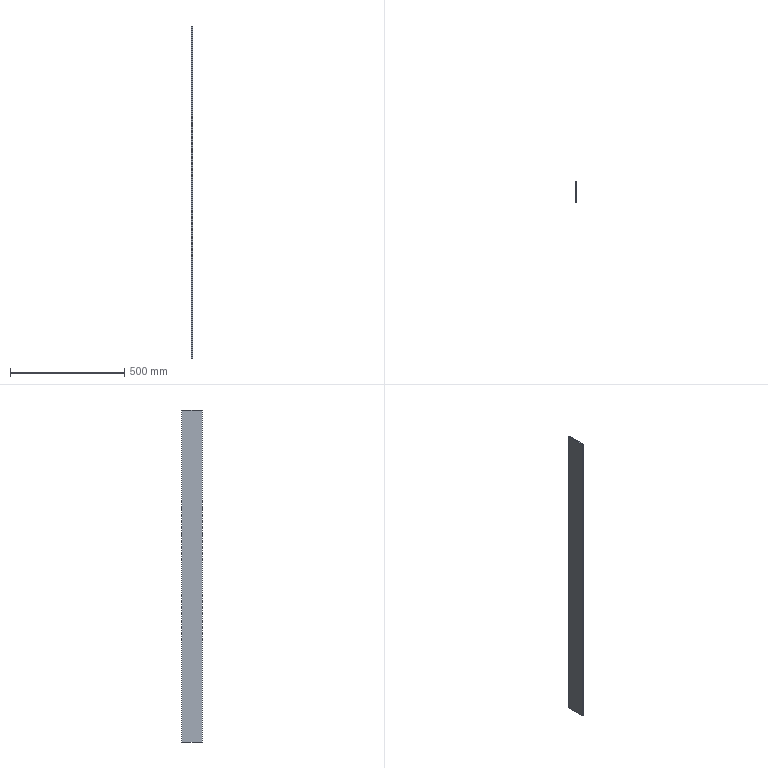Part | STEP file | _30001 | 1 solid | 6 faces | box 6 x 88 x 1450 mm | volume 765600 mm3 | plane 6
STEP:
#1=CARTESIAN_POINT('',(50.,-6.,725.));
#2=VERTEX_POINT('',#1);
#3=CARTESIAN_POINT('',(44.,-6.,725.));
#4=VERTEX_POINT('',#3);
#5=CARTESIAN_POINT('',(50.,-6.,725.));
#6=DIRECTION('',(-1.,0.,0.));
#7=VECTOR('',#6,1000.);
#8=LINE('',#5,#7);
#9=EDGE_CURVE('',#2,#4,#8,.T.);
#10=ORIENTED_EDGE('',*,*,#9,.T.);
#11=CARTESIAN_POINT('',(44.,-94.,725.));
#12=VERTEX_POINT('',#11);
#13=CARTESIAN_POINT('',(44.,-6.,725.));
#14=DIRECTION('',(0.,-1.,0.));
#15=VECTOR('',#14,1000.);
#16=LINE('',#13,#15);
#17=EDGE_CURVE('',#4,#12,#16,.T.);
#18=ORIENTED_EDGE('',*,*,#17,.T.);
#19=CARTESIAN_POINT('',(50.,-94.,725.));
#20=VERTEX_POINT('',#19);
#21=CARTESIAN_POINT('',(44.,-94.,725.));
#22=DIRECTION('',(1.,0.,0.));
#23=VECTOR('',#22,1000.);
#24=LINE('',#21,#23);
#25=EDGE_CURVE('',#12,#20,#24,.T.);
#26=ORIENTED_EDGE('',*,*,#25,.T.);
#27=CARTESIAN_POINT('',(50.,-6.,725.));
#28=DIRECTION('',(0.,-1.,0.));
#29=VECTOR('',#28,1000.);
#30=LINE('',#27,#29);
#31=EDGE_CURVE('',#2,#20,#30,.T.);
#32=ORIENTED_EDGE('',*,*,#31,.F.);
#33=EDGE_LOOP('',(#10,#18,#26,#32));
#34=FACE_OUTER_BOUND('',#33,.T.);
#35=CARTESIAN_POINT('',(0.,0.,725.));
#36=DIRECTION('',(0.,0.,-1.));
#37=DIRECTION('',(0.,-1.,0.));
#38=AXIS2_PLACEMENT_3D('',#35,#36,#37);
#39=PLANE('',#38);
#40=ADVANCED_FACE('',(#34),#39,.F.);
#41=CARTESIAN_POINT('',(44.,-6.,-725.));
#42=VERTEX_POINT('',#41);
#43=CARTESIAN_POINT('',(44.,-6.,-725.));
#44=DIRECTION('',(0.,0.,1.));
#45=VECTOR('',#44,1000.);
#46=LINE('',#43,#45);
#47=EDGE_CURVE('',#42,#4,#46,.T.);
#48=ORIENTED_EDGE('',*,*,#47,.T.);
#49=ORIENTED_EDGE('',*,*,#9,.F.);
#50=CARTESIAN_POINT('',(50.,-6.,-725.));
#51=VERTEX_POINT('',#50);
#52=CARTESIAN_POINT('',(50.,-6.,-725.));
#53=DIRECTION('',(0.,0.,1.));
#54=VECTOR('',#53,1000.);
#55=LINE('',#52,#54);
#56=EDGE_CURVE('',#51,#2,#55,.T.);
#57=ORIENTED_EDGE('',*,*,#56,.F.);
#58=CARTESIAN_POINT('',(50.,-6.,-725.));
#59=DIRECTION('',(-1.,0.,0.));
#60=VECTOR('',#59,1000.);
#61=LINE('',#58,#60);
#62=EDGE_CURVE('',#51,#42,#61,.T.);
#63=ORIENTED_EDGE('',*,*,#62,.T.);
#64=EDGE_LOOP('',(#48,#49,#57,#63));
#65=FACE_OUTER_BOUND('',#64,.T.);
#66=CARTESIAN_POINT('',(44.,-6.,725.));
#67=DIRECTION('',(0.,1.,0.));
#68=DIRECTION('',(1.,0.,0.));
#69=AXIS2_PLACEMENT_3D('',#66,#67,#68);
#70=PLANE('',#69);
#71=ADVANCED_FACE('',(#65),#70,.T.);
#72=CARTESIAN_POINT('',(44.,-94.,-725.));
#73=VERTEX_POINT('',#72);
#74=CARTESIAN_POINT('',(44.,-94.,-725.));
#75=DIRECTION('',(0.,0.,1.));
#76=VECTOR('',#75,1000.);
#77=LINE('',#74,#76);
#78=EDGE_CURVE('',#73,#12,#77,.T.);
#79=ORIENTED_EDGE('',*,*,#78,.T.);
#80=ORIENTED_EDGE('',*,*,#17,.F.);
#81=ORIENTED_EDGE('',*,*,#47,.F.);
#82=CARTESIAN_POINT('',(44.,-6.,-725.));
#83=DIRECTION('',(0.,-1.,0.));
#84=VECTOR('',#83,1000.);
#85=LINE('',#82,#84);
#86=EDGE_CURVE('',#42,#73,#85,.T.);
#87=ORIENTED_EDGE('',*,*,#86,.T.);
#88=EDGE_LOOP('',(#79,#80,#81,#87));
#89=FACE_OUTER_BOUND('',#88,.T.);
#90=CARTESIAN_POINT('',(44.,-94.,725.));
#91=DIRECTION('',(-1.,0.,0.));
#92=DIRECTION('',(0.,0.,1.));
#93=AXIS2_PLACEMENT_3D('',#90,#91,#92);
#94=PLANE('',#93);
#95=ADVANCED_FACE('',(#89),#94,.T.);
#96=CARTESIAN_POINT('',(50.,-94.,-725.));
#97=VERTEX_POINT('',#96);
#98=CARTESIAN_POINT('',(50.,-94.,-725.));
#99=DIRECTION('',(0.,0.,1.));
#100=VECTOR('',#99,1000.);
#101=LINE('',#98,#100);
#102=EDGE_CURVE('',#97,#20,#101,.T.);
#103=ORIENTED_EDGE('',*,*,#102,.T.);
#104=ORIENTED_EDGE('',*,*,#25,.F.);
#105=ORIENTED_EDGE('',*,*,#78,.F.);
#106=CARTESIAN_POINT('',(44.,-94.,-725.));
#107=DIRECTION('',(1.,0.,0.));
#108=VECTOR('',#107,1000.);
#109=LINE('',#106,#108);
#110=EDGE_CURVE('',#73,#97,#109,.T.);
#111=ORIENTED_EDGE('',*,*,#110,.T.);
#112=EDGE_LOOP('',(#103,#104,#105,#111));
#113=FACE_OUTER_BOUND('',#112,.T.);
#114=CARTESIAN_POINT('',(50.,-94.,725.));
#115=DIRECTION('',(0.,-1.,0.));
#116=DIRECTION('',(0.,0.,-1.));
#117=AXIS2_PLACEMENT_3D('',#114,#115,#116);
#118=PLANE('',#117);
#119=ADVANCED_FACE('',(#113),#118,.T.);
#120=ORIENTED_EDGE('',*,*,#56,.T.);
#121=ORIENTED_EDGE('',*,*,#31,.T.);
#122=ORIENTED_EDGE('',*,*,#102,.F.);
#123=CARTESIAN_POINT('',(50.,-6.,-725.));
#124=DIRECTION('',(0.,-1.,0.));
#125=VECTOR('',#124,1000.);
#126=LINE('',#123,#125);
#127=EDGE_CURVE('',#51,#97,#126,.T.);
#128=ORIENTED_EDGE('',*,*,#127,.F.);
#129=EDGE_LOOP('',(#120,#121,#122,#128));
#130=FACE_OUTER_BOUND('',#129,.T.);
#131=CARTESIAN_POINT('',(50.,-94.,725.));
#132=DIRECTION('',(-1.,0.,0.));
#133=DIRECTION('',(0.,0.,1.));
#134=AXIS2_PLACEMENT_3D('',#131,#132,#133);
#135=PLANE('',#134);
#136=ADVANCED_FACE('',(#130),#135,.F.);
#137=ORIENTED_EDGE('',*,*,#110,.F.);
#138=ORIENTED_EDGE('',*,*,#86,.F.);
#139=ORIENTED_EDGE('',*,*,#62,.F.);
#140=ORIENTED_EDGE('',*,*,#127,.T.);
#141=EDGE_LOOP('',(#137,#138,#139,#140));
#142=FACE_OUTER_BOUND('',#141,.T.);
#143=CARTESIAN_POINT('',(0.,0.,-725.));
#144=DIRECTION('',(0.,0.,-1.));
#145=DIRECTION('',(0.,-1.,0.));
#146=AXIS2_PLACEMENT_3D('',#143,#144,#145);
#147=PLANE('',#146);
#148=ADVANCED_FACE('',(#142),#147,.T.);
#149=CLOSED_SHELL('',(#40,#71,#95,#119,#136,#148));
#150=MANIFOLD_SOLID_BREP('',#149);
#151=CARTESIAN_POINT('',(0.,0.,0.));
#152=DIRECTION('',(0.,0.,1.));
#153=DIRECTION('',(1.,0.,0.));
#154=AXIS2_PLACEMENT_3D('',#151,#152,#153);
#155=(LENGTH_UNIT()NAMED_UNIT(*)SI_UNIT(.MILLI.,.METRE.));
#156=UNCERTAINTY_MEASURE_WITH_UNIT(LENGTH_MEASURE(0.00001),#155,'','');
#157=(NAMED_UNIT(*)PLANE_ANGLE_UNIT()SI_UNIT($,.RADIAN.));
#158=(NAMED_UNIT(*)SI_UNIT($,.STERADIAN.)SOLID_ANGLE_UNIT());
#159=(GEOMETRIC_REPRESENTATION_CONTEXT(3)GLOBAL_UNCERTAINTY_ASSIGNED_CONTEXT((#156))GLOBAL_UNIT_ASSIGNED_CONTEXT((#155,#157,#158))REPRESENTATION_CONTEXT('',''));
#160=ADVANCED_BREP_SHAPE_REPRESENTATION('',(#150,#154),#159);